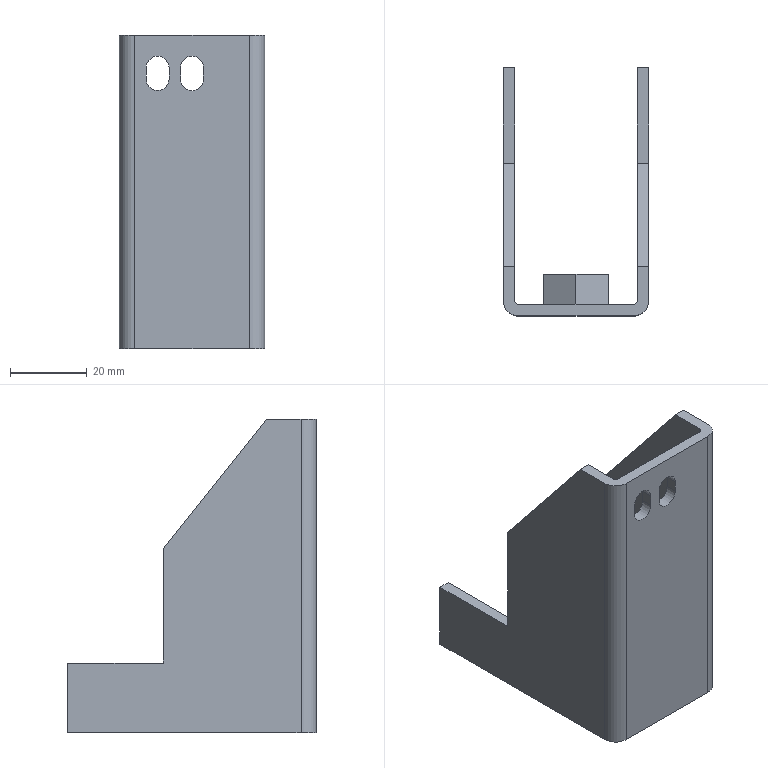Part | NX | features EXTRUDE 4, DATUM_CSYS 3, SKETCH 3, EXTRACT_DATUM_PLANE 1, UNITE 1 | 1 solid | 37 faces | box 38 x 65 x 82 mm | volume 28298 mm3 | plane 28 | cylinder 9 | commonest cylinder face diameters 6 x4 2 x2 8 x2 8.5 x1
STEP:
#1=CARTESIAN_POINT('',(-3.,-29.5,58.5));
#2=VERTEX_POINT('',#1);
#3=CARTESIAN_POINT('',(-3.,-29.5,61.5));
#4=VERTEX_POINT('',#3);
#5=CARTESIAN_POINT('',(-3.,-29.5,58.5));
#6=DIRECTION('',(0.,0.,1.));
#7=VECTOR('',#6,1000.);
#8=LINE('',#5,#7);
#9=EDGE_CURVE('',#2,#4,#8,.T.);
#10=ORIENTED_EDGE('',*,*,#9,.F.);
#11=CARTESIAN_POINT('',(3.,-29.5,58.5));
#12=VERTEX_POINT('',#11);
#13=CARTESIAN_POINT('',(0.,-29.5,58.5));
#14=DIRECTION('',(0.,1.,0.));
#15=DIRECTION('',(-1.,0.,0.));
#16=AXIS2_PLACEMENT_3D('',#13,#14,#15);
#17=CIRCLE('',#16,3.);
#18=EDGE_CURVE('',#12,#2,#17,.T.);
#19=ORIENTED_EDGE('',*,*,#18,.F.);
#20=CARTESIAN_POINT('',(3.,-29.5,61.5));
#21=VERTEX_POINT('',#20);
#22=CARTESIAN_POINT('',(3.,-29.5,61.5));
#23=DIRECTION('',(0.,0.,-1.));
#24=VECTOR('',#23,1000.);
#25=LINE('',#22,#24);
#26=EDGE_CURVE('',#21,#12,#25,.T.);
#27=ORIENTED_EDGE('',*,*,#26,.F.);
#28=CARTESIAN_POINT('',(0.,-29.5,61.5));
#29=DIRECTION('',(0.,1.,0.));
#30=DIRECTION('',(1.,0.,0.));
#31=AXIS2_PLACEMENT_3D('',#28,#29,#30);
#32=CIRCLE('',#31,3.);
#33=EDGE_CURVE('',#4,#21,#32,.T.);
#34=ORIENTED_EDGE('',*,*,#33,.F.);
#35=EDGE_LOOP('',(#10,#19,#27,#34));
#36=FACE_BOUND('',#35,.T.);
#37=CARTESIAN_POINT('',(-12.,-29.5,58.5));
#38=VERTEX_POINT('',#37);
#39=CARTESIAN_POINT('',(-12.,-29.5,61.5));
#40=VERTEX_POINT('',#39);
#41=CARTESIAN_POINT('',(-12.,-29.5,58.5));
#42=DIRECTION('',(0.,0.,1.));
#43=VECTOR('',#42,1000.);
#44=LINE('',#41,#43);
#45=EDGE_CURVE('',#38,#40,#44,.T.);
#46=ORIENTED_EDGE('',*,*,#45,.F.);
#47=CARTESIAN_POINT('',(-6.,-29.5,58.5));
#48=VERTEX_POINT('',#47);
#49=CARTESIAN_POINT('',(-9.,-29.5,58.5));
#50=DIRECTION('',(0.,1.,0.));
#51=DIRECTION('',(-1.,0.,0.));
#52=AXIS2_PLACEMENT_3D('',#49,#50,#51);
#53=CIRCLE('',#52,3.);
#54=EDGE_CURVE('',#48,#38,#53,.T.);
#55=ORIENTED_EDGE('',*,*,#54,.F.);
#56=CARTESIAN_POINT('',(-6.,-29.5,61.5));
#57=VERTEX_POINT('',#56);
#58=CARTESIAN_POINT('',(-6.,-29.5,61.5));
#59=DIRECTION('',(0.,0.,-1.));
#60=VECTOR('',#59,1000.);
#61=LINE('',#58,#60);
#62=EDGE_CURVE('',#57,#48,#61,.T.);
#63=ORIENTED_EDGE('',*,*,#62,.F.);
#64=CARTESIAN_POINT('',(-9.,-29.5,61.5));
#65=DIRECTION('',(0.,1.,0.));
#66=DIRECTION('',(1.,0.,0.));
#67=AXIS2_PLACEMENT_3D('',#64,#65,#66);
#68=CIRCLE('',#67,3.);
#69=EDGE_CURVE('',#40,#57,#68,.T.);
#70=ORIENTED_EDGE('',*,*,#69,.F.);
#71=EDGE_LOOP('',(#46,#55,#63,#70));
#72=FACE_BOUND('',#71,.T.);
#73=CARTESIAN_POINT('',(15.,-29.5,70.));
#74=VERTEX_POINT('',#73);
#75=CARTESIAN_POINT('',(-15.,-29.5,70.));
#76=VERTEX_POINT('',#75);
#77=CARTESIAN_POINT('',(15.,-29.5,70.));
#78=DIRECTION('',(-1.,0.,0.));
#79=VECTOR('',#78,1000.);
#80=LINE('',#77,#79);
#81=EDGE_CURVE('',#74,#76,#80,.T.);
#82=ORIENTED_EDGE('',*,*,#81,.F.);
#83=CARTESIAN_POINT('',(15.,-29.5,-12.));
#84=VERTEX_POINT('',#83);
#85=CARTESIAN_POINT('',(15.,-29.5,-12.));
#86=DIRECTION('',(0.,0.,1.));
#87=VECTOR('',#86,1000.);
#88=LINE('',#85,#87);
#89=EDGE_CURVE('',#84,#74,#88,.T.);
#90=ORIENTED_EDGE('',*,*,#89,.F.);
#91=CARTESIAN_POINT('',(-15.,-29.5,-12.));
#92=VERTEX_POINT('',#91);
#93=CARTESIAN_POINT('',(15.,-29.5,-12.));
#94=DIRECTION('',(-1.,0.,0.));
#95=VECTOR('',#94,1000.);
#96=LINE('',#93,#95);
#97=EDGE_CURVE('',#84,#92,#96,.T.);
#98=ORIENTED_EDGE('',*,*,#97,.T.);
#99=CARTESIAN_POINT('',(-15.,-29.5,-12.));
#100=DIRECTION('',(0.,0.,1.));
#101=VECTOR('',#100,1000.);
#102=LINE('',#99,#101);
#103=EDGE_CURVE('',#92,#76,#102,.T.);
#104=ORIENTED_EDGE('',*,*,#103,.T.);
#105=EDGE_LOOP('',(#82,#90,#98,#104));
#106=FACE_BOUND('',#105,.T.);
#107=CARTESIAN_POINT('',(8.5,-29.5,4.907));
#108=VERTEX_POINT('',#107);
#109=CARTESIAN_POINT('',(8.5,-29.5,-4.907));
#110=VERTEX_POINT('',#109);
#111=CARTESIAN_POINT('',(8.5,-29.5,4.907));
#112=DIRECTION('',(0.,0.,-1.));
#113=VECTOR('',#112,1000.);
#114=LINE('',#111,#113);
#115=EDGE_CURVE('',#108,#110,#114,.T.);
#116=ORIENTED_EDGE('',*,*,#115,.F.);
#117=CARTESIAN_POINT('',(0.,-29.5,9.815));
#118=VERTEX_POINT('',#117);
#119=CARTESIAN_POINT('',(0.,-29.5,9.815));
#120=DIRECTION('',(0.866,0.,-0.5));
#121=VECTOR('',#120,1000.);
#122=LINE('',#119,#121);
#123=EDGE_CURVE('',#118,#108,#122,.T.);
#124=ORIENTED_EDGE('',*,*,#123,.F.);
#125=CARTESIAN_POINT('',(-8.5,-29.5,4.907));
#126=VERTEX_POINT('',#125);
#127=CARTESIAN_POINT('',(-8.5,-29.5,4.907));
#128=DIRECTION('',(0.866,0.,0.5));
#129=VECTOR('',#128,1000.);
#130=LINE('',#127,#129);
#131=EDGE_CURVE('',#126,#118,#130,.T.);
#132=ORIENTED_EDGE('',*,*,#131,.F.);
#133=CARTESIAN_POINT('',(-8.5,-29.5,-4.907));
#134=VERTEX_POINT('',#133);
#135=CARTESIAN_POINT('',(-8.5,-29.5,-4.907));
#136=DIRECTION('',(0.,0.,1.));
#137=VECTOR('',#136,1000.);
#138=LINE('',#135,#137);
#139=EDGE_CURVE('',#134,#126,#138,.T.);
#140=ORIENTED_EDGE('',*,*,#139,.F.);
#141=CARTESIAN_POINT('',(0.,-29.5,-9.815));
#142=VERTEX_POINT('',#141);
#143=CARTESIAN_POINT('',(0.,-29.5,-9.815));
#144=DIRECTION('',(-0.866,0.,0.5));
#145=VECTOR('',#144,1000.);
#146=LINE('',#143,#145);
#147=EDGE_CURVE('',#142,#134,#146,.T.);
#148=ORIENTED_EDGE('',*,*,#147,.F.);
#149=CARTESIAN_POINT('',(8.5,-29.5,-4.907));
#150=DIRECTION('',(-0.866,0.,-0.5));
#151=VECTOR('',#150,1000.);
#152=LINE('',#149,#151);
#153=EDGE_CURVE('',#110,#142,#152,.T.);
#154=ORIENTED_EDGE('',*,*,#153,.F.);
#155=EDGE_LOOP('',(#116,#124,#132,#140,#148,#154));
#156=FACE_BOUND('',#155,.T.);
#157=CARTESIAN_POINT('',(15.,-29.5,-12.));
#158=DIRECTION('',(0.,1.,0.));
#159=DIRECTION('',(0.,0.,1.));
#160=AXIS2_PLACEMENT_3D('',#157,#158,#159);
#161=PLANE('',#160);
#162=ADVANCED_FACE('',(#36,#72,#106,#156),#161,.T.);
#163=CARTESIAN_POINT('',(-19.,-28.5,70.));
#164=VERTEX_POINT('',#163);
#165=CARTESIAN_POINT('',(-15.,-32.5,70.));
#166=VERTEX_POINT('',#165);
#167=CARTESIAN_POINT('',(-15.,-28.5,70.));
#168=DIRECTION('',(0.,0.,1.));
#169=DIRECTION('',(-1.,0.,0.));
#170=AXIS2_PLACEMENT_3D('',#167,#168,#169);
#171=CIRCLE('',#170,4.);
#172=EDGE_CURVE('',#164,#166,#171,.T.);
#173=ORIENTED_EDGE('',*,*,#172,.F.);
#174=CARTESIAN_POINT('',(-19.,-28.5,-12.));
#175=VERTEX_POINT('',#174);
#176=CARTESIAN_POINT('',(-19.,-28.5,-12.));
#177=DIRECTION('',(0.,0.,1.));
#178=VECTOR('',#177,1000.);
#179=LINE('',#176,#178);
#180=EDGE_CURVE('',#175,#164,#179,.T.);
#181=ORIENTED_EDGE('',*,*,#180,.F.);
#182=CARTESIAN_POINT('',(-15.,-32.5,-12.));
#183=VERTEX_POINT('',#182);
#184=CARTESIAN_POINT('',(-15.,-28.5,-12.));
#185=DIRECTION('',(0.,0.,1.));
#186=DIRECTION('',(-1.,0.,0.));
#187=AXIS2_PLACEMENT_3D('',#184,#185,#186);
#188=CIRCLE('',#187,4.);
#189=EDGE_CURVE('',#175,#183,#188,.T.);
#190=ORIENTED_EDGE('',*,*,#189,.T.);
#191=CARTESIAN_POINT('',(-15.,-32.5,-12.));
#192=DIRECTION('',(0.,0.,1.));
#193=VECTOR('',#192,1000.);
#194=LINE('',#191,#193);
#195=EDGE_CURVE('',#183,#166,#194,.T.);
#196=ORIENTED_EDGE('',*,*,#195,.T.);
#197=EDGE_LOOP('',(#173,#181,#190,#196));
#198=FACE_BOUND('',#197,.T.);
#199=CARTESIAN_POINT('',(-15.,-28.5,-12.));
#200=DIRECTION('',(0.,0.,1.));
#201=DIRECTION('',(1.,0.,0.));
#202=AXIS2_PLACEMENT_3D('',#199,#200,#201);
#203=CYLINDRICAL_SURFACE('',#202,4.);
#204=ADVANCED_FACE('',(#198),#203,.T.);
#205=CARTESIAN_POINT('',(-3.,-32.5,61.5));
#206=VERTEX_POINT('',#205);
#207=CARTESIAN_POINT('',(-3.,-32.5,58.5));
#208=VERTEX_POINT('',#207);
#209=CARTESIAN_POINT('',(-3.,-32.5,-12.));
#210=DIRECTION('',(0.,0.,-1.));
#211=VECTOR('',#210,1000.);
#212=LINE('',#209,#211);
#213=EDGE_CURVE('',#206,#208,#212,.T.);
#214=ORIENTED_EDGE('',*,*,#213,.F.);
#215=CARTESIAN_POINT('',(3.,-32.5,61.5));
#216=VERTEX_POINT('',#215);
#217=CARTESIAN_POINT('',(0.,-32.5,61.5));
#218=DIRECTION('',(0.,-1.,0.));
#219=DIRECTION('',(0.,0.,-1.));
#220=AXIS2_PLACEMENT_3D('',#217,#218,#219);
#221=CIRCLE('',#220,3.);
#222=EDGE_CURVE('',#216,#206,#221,.T.);
#223=ORIENTED_EDGE('',*,*,#222,.F.);
#224=CARTESIAN_POINT('',(3.,-32.5,58.5));
#225=VERTEX_POINT('',#224);
#226=CARTESIAN_POINT('',(3.,-32.5,-12.));
#227=DIRECTION('',(0.,0.,1.));
#228=VECTOR('',#227,1000.);
#229=LINE('',#226,#228);
#230=EDGE_CURVE('',#225,#216,#229,.T.);
#231=ORIENTED_EDGE('',*,*,#230,.F.);
#232=CARTESIAN_POINT('',(0.,-32.5,58.5));
#233=DIRECTION('',(0.,-1.,0.));
#234=DIRECTION('',(0.,0.,-1.));
#235=AXIS2_PLACEMENT_3D('',#232,#233,#234);
#236=CIRCLE('',#235,3.);
#237=EDGE_CURVE('',#208,#225,#236,.T.);
#238=ORIENTED_EDGE('',*,*,#237,.F.);
#239=EDGE_LOOP('',(#214,#223,#231,#238));
#240=FACE_BOUND('',#239,.T.);
#241=CARTESIAN_POINT('',(-12.,-32.5,61.5));
#242=VERTEX_POINT('',#241);
#243=CARTESIAN_POINT('',(-12.,-32.5,58.5));
#244=VERTEX_POINT('',#243);
#245=CARTESIAN_POINT('',(-12.,-32.5,-12.));
#246=DIRECTION('',(0.,0.,-1.));
#247=VECTOR('',#246,1000.);
#248=LINE('',#245,#247);
#249=EDGE_CURVE('',#242,#244,#248,.T.);
#250=ORIENTED_EDGE('',*,*,#249,.F.);
#251=CARTESIAN_POINT('',(-6.,-32.5,61.5));
#252=VERTEX_POINT('',#251);
#253=CARTESIAN_POINT('',(-9.,-32.5,61.5));
#254=DIRECTION('',(0.,-1.,0.));
#255=DIRECTION('',(0.,0.,-1.));
#256=AXIS2_PLACEMENT_3D('',#253,#254,#255);
#257=CIRCLE('',#256,3.);
#258=EDGE_CURVE('',#252,#242,#257,.T.);
#259=ORIENTED_EDGE('',*,*,#258,.F.);
#260=CARTESIAN_POINT('',(-6.,-32.5,58.5));
#261=VERTEX_POINT('',#260);
#262=CARTESIAN_POINT('',(-6.,-32.5,-12.));
#263=DIRECTION('',(0.,0.,1.));
#264=VECTOR('',#263,1000.);
#265=LINE('',#262,#264);
#266=EDGE_CURVE('',#261,#252,#265,.T.);
#267=ORIENTED_EDGE('',*,*,#266,.F.);
#268=CARTESIAN_POINT('',(-9.,-32.5,58.5));
#269=DIRECTION('',(0.,-1.,0.));
#270=DIRECTION('',(0.,0.,-1.));
#271=AXIS2_PLACEMENT_3D('',#268,#269,#270);
#272=CIRCLE('',#271,3.);
#273=EDGE_CURVE('',#244,#261,#272,.T.);
#274=ORIENTED_EDGE('',*,*,#273,.F.);
#275=EDGE_LOOP('',(#250,#259,#267,#274));
#276=FACE_BOUND('',#275,.T.);
#277=CARTESIAN_POINT('',(15.,-32.5,70.));
#278=VERTEX_POINT('',#277);
#279=CARTESIAN_POINT('',(-15.,-32.5,70.));
#280=DIRECTION('',(1.,0.,0.));
#281=VECTOR('',#280,1000.);
#282=LINE('',#279,#281);
#283=EDGE_CURVE('',#166,#278,#282,.T.);
#284=ORIENTED_EDGE('',*,*,#283,.F.);
#285=ORIENTED_EDGE('',*,*,#195,.F.);
#286=CARTESIAN_POINT('',(15.,-32.5,-12.));
#287=VERTEX_POINT('',#286);
#288=CARTESIAN_POINT('',(-15.,-32.5,-12.));
#289=DIRECTION('',(1.,0.,0.));
#290=VECTOR('',#289,1000.);
#291=LINE('',#288,#290);
#292=EDGE_CURVE('',#183,#287,#291,.T.);
#293=ORIENTED_EDGE('',*,*,#292,.T.);
#294=CARTESIAN_POINT('',(15.,-32.5,-12.));
#295=DIRECTION('',(0.,0.,1.));
#296=VECTOR('',#295,1000.);
#297=LINE('',#294,#296);
#298=EDGE_CURVE('',#287,#278,#297,.T.);
#299=ORIENTED_EDGE('',*,*,#298,.T.);
#300=EDGE_LOOP('',(#284,#285,#293,#299));
#301=FACE_BOUND('',#300,.T.);
#302=CARTESIAN_POINT('',(-15.,-32.5,-12.));
#303=DIRECTION('',(0.,-1.,0.));
#304=DIRECTION('',(0.,0.,-1.));
#305=AXIS2_PLACEMENT_3D('',#302,#303,#304);
#306=PLANE('',#305);
#307=ADVANCED_FACE('',(#240,#276,#301),#306,.T.);
#308=CARTESIAN_POINT('',(19.,-28.5,70.));
#309=VERTEX_POINT('',#308);
#310=CARTESIAN_POINT('',(15.,-28.5,70.));
#311=DIRECTION('',(0.,0.,1.));
#312=DIRECTION('',(0.,-1.,0.));
#313=AXIS2_PLACEMENT_3D('',#310,#311,#312);
#314=CIRCLE('',#313,4.);
#315=EDGE_CURVE('',#278,#309,#314,.T.);
#316=ORIENTED_EDGE('',*,*,#315,.F.);
#317=ORIENTED_EDGE('',*,*,#298,.F.);
#318=CARTESIAN_POINT('',(19.,-28.5,-12.));
#319=VERTEX_POINT('',#318);
#320=CARTESIAN_POINT('',(15.,-28.5,-12.));
#321=DIRECTION('',(0.,0.,1.));
#322=DIRECTION('',(0.,-1.,0.));
#323=AXIS2_PLACEMENT_3D('',#320,#321,#322);
#324=CIRCLE('',#323,4.);
#325=EDGE_CURVE('',#287,#319,#324,.T.);
#326=ORIENTED_EDGE('',*,*,#325,.T.);
#327=CARTESIAN_POINT('',(19.,-28.5,-12.));
#328=DIRECTION('',(0.,0.,1.));
#329=VECTOR('',#328,1000.);
#330=LINE('',#327,#329);
#331=EDGE_CURVE('',#319,#309,#330,.T.);
#332=ORIENTED_EDGE('',*,*,#331,.T.);
#333=EDGE_LOOP('',(#316,#317,#326,#332));
#334=FACE_BOUND('',#333,.T.);
#335=CARTESIAN_POINT('',(15.,-28.5,-12.));
#336=DIRECTION('',(0.,0.,1.));
#337=DIRECTION('',(1.,0.,0.));
#338=AXIS2_PLACEMENT_3D('',#335,#336,#337);
#339=CYLINDRICAL_SURFACE('',#338,4.);
#340=ADVANCED_FACE('',(#334),#339,.T.);
#341=CARTESIAN_POINT('',(19.,7.5,6.25));
#342=VERTEX_POINT('',#341);
#343=CARTESIAN_POINT('',(19.,32.5,6.25));
#344=VERTEX_POINT('',#343);
#345=CARTESIAN_POINT('',(19.,7.5,6.25));
#346=DIRECTION('',(0.,1.,0.));
#347=VECTOR('',#346,1000.);
#348=LINE('',#345,#347);
#349=EDGE_CURVE('',#342,#344,#348,.T.);
#350=ORIENTED_EDGE('',*,*,#349,.F.);
#351=CARTESIAN_POINT('',(19.,7.5,36.25));
#352=VERTEX_POINT('',#351);
#353=CARTESIAN_POINT('',(19.,7.5,-12.));
#354=DIRECTION('',(0.,0.,-1.));
#355=VECTOR('',#354,1000.);
#356=LINE('',#353,#355);
#357=EDGE_CURVE('',#352,#342,#356,.T.);
#358=ORIENTED_EDGE('',*,*,#357,.F.);
#359=CARTESIAN_POINT('',(19.,-19.5,70.));
#360=VERTEX_POINT('',#359);
#361=CARTESIAN_POINT('',(19.,31.037,6.829));
#362=DIRECTION('',(0.,0.6247,-0.7809));
#363=VECTOR('',#362,1000.);
#364=LINE('',#361,#363);
#365=EDGE_CURVE('',#360,#352,#364,.T.);
#366=ORIENTED_EDGE('',*,*,#365,.F.);
#367=CARTESIAN_POINT('',(19.,7.5,70.));
#368=DIRECTION('',(0.,1.,0.));
#369=VECTOR('',#368,1000.);
#370=LINE('',#367,#369);
#371=EDGE_CURVE('',#309,#360,#370,.T.);
#372=ORIENTED_EDGE('',*,*,#371,.F.);
#373=ORIENTED_EDGE('',*,*,#331,.F.);
#374=CARTESIAN_POINT('',(19.,32.5,-12.));
#375=VERTEX_POINT('',#374);
#376=CARTESIAN_POINT('',(19.,-28.5,-12.));
#377=DIRECTION('',(0.,1.,0.));
#378=VECTOR('',#377,1000.);
#379=LINE('',#376,#378);
#380=EDGE_CURVE('',#319,#375,#379,.T.);
#381=ORIENTED_EDGE('',*,*,#380,.T.);
#382=CARTESIAN_POINT('',(19.,32.5,-12.));
#383=DIRECTION('',(0.,0.,1.));
#384=VECTOR('',#383,1000.);
#385=LINE('',#382,#384);
#386=EDGE_CURVE('',#375,#344,#385,.T.);
#387=ORIENTED_EDGE('',*,*,#386,.T.);
#388=EDGE_LOOP('',(#350,#358,#366,#372,#373,#381,#387));
#389=FACE_BOUND('',#388,.T.);
#390=CARTESIAN_POINT('',(19.,7.5,-12.));
#391=DIRECTION('',(1.,0.,0.));
#392=DIRECTION('',(0.,0.,-1.));
#393=AXIS2_PLACEMENT_3D('',#390,#391,#392);
#394=PLANE('',#393);
#395=ADVANCED_FACE('',(#389),#394,.T.);
#396=CARTESIAN_POINT('',(16.,32.5,6.25));
#397=VERTEX_POINT('',#396);
#398=CARTESIAN_POINT('',(19.,32.5,6.25));
#399=DIRECTION('',(-1.,0.,0.));
#400=VECTOR('',#399,1000.);
#401=LINE('',#398,#400);
#402=EDGE_CURVE('',#344,#397,#401,.T.);
#403=ORIENTED_EDGE('',*,*,#402,.F.);
#404=ORIENTED_EDGE('',*,*,#386,.F.);
#405=CARTESIAN_POINT('',(16.,32.5,-12.));
#406=VERTEX_POINT('',#405);
#407=CARTESIAN_POINT('',(19.,32.5,-12.));
#408=DIRECTION('',(-1.,0.,0.));
#409=VECTOR('',#408,1000.);
#410=LINE('',#407,#409);
#411=EDGE_CURVE('',#375,#406,#410,.T.);
#412=ORIENTED_EDGE('',*,*,#411,.T.);
#413=CARTESIAN_POINT('',(16.,32.5,-12.));
#414=DIRECTION('',(0.,0.,1.));
#415=VECTOR('',#414,1000.);
#416=LINE('',#413,#415);
#417=EDGE_CURVE('',#406,#397,#416,.T.);
#418=ORIENTED_EDGE('',*,*,#417,.T.);
#419=EDGE_LOOP('',(#403,#404,#412,#418));
#420=FACE_BOUND('',#419,.T.);
#421=CARTESIAN_POINT('',(19.,32.5,-12.));
#422=DIRECTION('',(0.,1.,0.));
#423=DIRECTION('',(0.,0.,1.));
#424=AXIS2_PLACEMENT_3D('',#421,#422,#423);
#425=PLANE('',#424);
#426=ADVANCED_FACE('',(#420),#425,.T.);
#427=CARTESIAN_POINT('',(16.,7.5,6.25));
#428=VERTEX_POINT('',#427);
#429=CARTESIAN_POINT('',(16.,-19.5,6.25));
#430=DIRECTION('',(0.,-1.,0.));
#431=VECTOR('',#430,1000.);
#432=LINE('',#429,#431);
#433=EDGE_CURVE('',#397,#428,#432,.T.);
#434=ORIENTED_EDGE('',*,*,#433,.F.);
#435=ORIENTED_EDGE('',*,*,#417,.F.);
#436=CARTESIAN_POINT('',(16.,-28.5,-12.));
#437=VERTEX_POINT('',#436);
#438=CARTESIAN_POINT('',(16.,32.5,-12.));
#439=DIRECTION('',(0.,-1.,0.));
#440=VECTOR('',#439,1000.);
#441=LINE('',#438,#440);
#442=EDGE_CURVE('',#406,#437,#441,.T.);
#443=ORIENTED_EDGE('',*,*,#442,.T.);
#444=CARTESIAN_POINT('',(16.,-28.5,70.));
#445=VERTEX_POINT('',#444);
#446=CARTESIAN_POINT('',(16.,-28.5,-12.));
#447=DIRECTION('',(0.,0.,1.));
#448=VECTOR('',#447,1000.);
#449=LINE('',#446,#448);
#450=EDGE_CURVE('',#437,#445,#449,.T.);
#451=ORIENTED_EDGE('',*,*,#450,.T.);
#452=CARTESIAN_POINT('',(16.,-19.5,70.));
#453=VERTEX_POINT('',#452);
#454=CARTESIAN_POINT('',(16.,-19.5,70.));
#455=DIRECTION('',(0.,-1.,0.));
#456=VECTOR('',#455,1000.);
#457=LINE('',#454,#456);
#458=EDGE_CURVE('',#453,#445,#457,.T.);
#459=ORIENTED_EDGE('',*,*,#458,.F.);
#460=CARTESIAN_POINT('',(16.,7.5,36.25));
#461=VERTEX_POINT('',#460);
#462=CARTESIAN_POINT('',(16.,20.5,20.));
#463=DIRECTION('',(0.,-0.6247,0.7809));
#464=VECTOR('',#463,1000.);
#465=LINE('',#462,#464);
#466=EDGE_CURVE('',#461,#453,#465,.T.);
#467=ORIENTED_EDGE('',*,*,#466,.F.);
#468=CARTESIAN_POINT('',(16.,7.5,-12.));
#469=DIRECTION('',(0.,0.,1.));
#470=VECTOR('',#469,1000.);
#471=LINE('',#468,#470);
#472=EDGE_CURVE('',#428,#461,#471,.T.);
#473=ORIENTED_EDGE('',*,*,#472,.F.);
#474=EDGE_LOOP('',(#434,#435,#443,#451,#459,#467,#473));
#475=FACE_BOUND('',#474,.T.);
#476=CARTESIAN_POINT('',(16.,-19.5,-12.));
#477=DIRECTION('',(-1.,0.,0.));
#478=DIRECTION('',(0.,0.,1.));
#479=AXIS2_PLACEMENT_3D('',#476,#477,#478);
#480=PLANE('',#479);
#481=ADVANCED_FACE('',(#475),#480,.T.);
#482=CARTESIAN_POINT('',(15.,-28.5,70.));
#483=DIRECTION('',(0.,0.,-1.));
#484=DIRECTION('',(1.,0.,0.));
#485=AXIS2_PLACEMENT_3D('',#482,#483,#484);
#486=CIRCLE('',#485,1.);
#487=EDGE_CURVE('',#445,#74,#486,.T.);
#488=ORIENTED_EDGE('',*,*,#487,.F.);
#489=ORIENTED_EDGE('',*,*,#450,.F.);
#490=CARTESIAN_POINT('',(15.,-28.5,-12.));
#491=DIRECTION('',(0.,0.,-1.));
#492=DIRECTION('',(1.,0.,0.));
#493=AXIS2_PLACEMENT_3D('',#490,#491,#492);
#494=CIRCLE('',#493,1.);
#495=EDGE_CURVE('',#437,#84,#494,.T.);
#496=ORIENTED_EDGE('',*,*,#495,.T.);
#497=ORIENTED_EDGE('',*,*,#89,.T.);
#498=EDGE_LOOP('',(#488,#489,#496,#497));
#499=FACE_BOUND('',#498,.T.);
#500=CARTESIAN_POINT('',(15.,-28.5,-12.));
#501=DIRECTION('',(0.,0.,1.));
#502=DIRECTION('',(1.,0.,0.));
#503=AXIS2_PLACEMENT_3D('',#500,#501,#502);
#504=CYLINDRICAL_SURFACE('',#503,1.);
#505=ADVANCED_FACE('',(#499),#504,.F.);
#506=CARTESIAN_POINT('',(-16.,-28.5,70.));
#507=VERTEX_POINT('',#506);
#508=CARTESIAN_POINT('',(-15.,-28.5,70.));
#509=DIRECTION('',(0.,0.,-1.));
#510=DIRECTION('',(0.,-1.,0.));
#511=AXIS2_PLACEMENT_3D('',#508,#509,#510);
#512=CIRCLE('',#511,1.);
#513=EDGE_CURVE('',#76,#507,#512,.T.);
#514=ORIENTED_EDGE('',*,*,#513,.F.);
#515=ORIENTED_EDGE('',*,*,#103,.F.);
#516=CARTESIAN_POINT('',(-16.,-28.5,-12.));
#517=VERTEX_POINT('',#516);
#518=CARTESIAN_POINT('',(-15.,-28.5,-12.));
#519=DIRECTION('',(0.,0.,-1.));
#520=DIRECTION('',(0.,-1.,0.));
#521=AXIS2_PLACEMENT_3D('',#518,#519,#520);
#522=CIRCLE('',#521,1.);
#523=EDGE_CURVE('',#92,#517,#522,.T.);
#524=ORIENTED_EDGE('',*,*,#523,.T.);
#525=CARTESIAN_POINT('',(-16.,-28.5,-12.));
#526=DIRECTION('',(0.,0.,1.));
#527=VECTOR('',#526,1000.);
#528=LINE('',#525,#527);
#529=EDGE_CURVE('',#517,#507,#528,.T.);
#530=ORIENTED_EDGE('',*,*,#529,.T.);
#531=EDGE_LOOP('',(#514,#515,#524,#530));
#532=FACE_BOUND('',#531,.T.);
#533=CARTESIAN_POINT('',(-15.,-28.5,-12.));
#534=DIRECTION('',(0.,0.,1.));
#535=DIRECTION('',(1.,0.,0.));
#536=AXIS2_PLACEMENT_3D('',#533,#534,#535);
#537=CYLINDRICAL_SURFACE('',#536,1.);
#538=ADVANCED_FACE('',(#532),#537,.F.);
#539=CARTESIAN_POINT('',(-16.,7.5,6.25));
#540=VERTEX_POINT('',#539);
#541=CARTESIAN_POINT('',(-16.,32.5,6.25));
#542=VERTEX_POINT('',#541);
#543=CARTESIAN_POINT('',(-16.,7.5,6.25));
#544=DIRECTION('',(0.,1.,0.));
#545=VECTOR('',#544,1000.);
#546=LINE('',#543,#545);
#547=EDGE_CURVE('',#540,#542,#546,.T.);
#548=ORIENTED_EDGE('',*,*,#547,.F.);
#549=CARTESIAN_POINT('',(-16.,7.5,36.25));
#550=VERTEX_POINT('',#549);
#551=CARTESIAN_POINT('',(-16.,7.5,-12.));
#552=DIRECTION('',(0.,0.,-1.));
#553=VECTOR('',#552,1000.);
#554=LINE('',#551,#553);
#555=EDGE_CURVE('',#550,#540,#554,.T.);
#556=ORIENTED_EDGE('',*,*,#555,.F.);
#557=CARTESIAN_POINT('',(-16.,-19.5,70.));
#558=VERTEX_POINT('',#557);
#559=CARTESIAN_POINT('',(-16.,31.037,6.829));
#560=DIRECTION('',(0.,0.6247,-0.7809));
#561=VECTOR('',#560,1000.);
#562=LINE('',#559,#561);
#563=EDGE_CURVE('',#558,#550,#562,.T.);
#564=ORIENTED_EDGE('',*,*,#563,.F.);
#565=CARTESIAN_POINT('',(-16.,7.5,70.));
#566=DIRECTION('',(0.,1.,0.));
#567=VECTOR('',#566,1000.);
#568=LINE('',#565,#567);
#569=EDGE_CURVE('',#507,#558,#568,.T.);
#570=ORIENTED_EDGE('',*,*,#569,.F.);
#571=ORIENTED_EDGE('',*,*,#529,.F.);
#572=CARTESIAN_POINT('',(-16.,32.5,-12.));
#573=VERTEX_POINT('',#572);
#574=CARTESIAN_POINT('',(-16.,-28.5,-12.));
#575=DIRECTION('',(0.,1.,0.));
#576=VECTOR('',#575,1000.);
#577=LINE('',#574,#576);
#578=EDGE_CURVE('',#517,#573,#577,.T.);
#579=ORIENTED_EDGE('',*,*,#578,.T.);
#580=CARTESIAN_POINT('',(-16.,32.5,-12.));
#581=DIRECTION('',(0.,0.,1.));
#582=VECTOR('',#581,1000.);
#583=LINE('',#580,#582);
#584=EDGE_CURVE('',#573,#542,#583,.T.);
#585=ORIENTED_EDGE('',*,*,#584,.T.);
#586=EDGE_LOOP('',(#548,#556,#564,#570,#571,#579,#585));
#587=FACE_BOUND('',#586,.T.);
#588=CARTESIAN_POINT('',(-16.,7.5,-12.));
#589=DIRECTION('',(1.,0.,0.));
#590=DIRECTION('',(0.,0.,-1.));
#591=AXIS2_PLACEMENT_3D('',#588,#589,#590);
#592=PLANE('',#591);
#593=ADVANCED_FACE('',(#587),#592,.T.);
#594=CARTESIAN_POINT('',(-19.,32.5,6.25));
#595=VERTEX_POINT('',#594);
#596=CARTESIAN_POINT('',(-16.,32.5,6.25));
#597=DIRECTION('',(-1.,0.,0.));
#598=VECTOR('',#597,1000.);
#599=LINE('',#596,#598);
#600=EDGE_CURVE('',#542,#595,#599,.T.);
#601=ORIENTED_EDGE('',*,*,#600,.F.);
#602=ORIENTED_EDGE('',*,*,#584,.F.);
#603=CARTESIAN_POINT('',(-19.,32.5,-12.));
#604=VERTEX_POINT('',#603);
#605=CARTESIAN_POINT('',(-16.,32.5,-12.));
#606=DIRECTION('',(-1.,0.,0.));
#607=VECTOR('',#606,1000.);
#608=LINE('',#605,#607);
#609=EDGE_CURVE('',#573,#604,#608,.T.);
#610=ORIENTED_EDGE('',*,*,#609,.T.);
#611=CARTESIAN_POINT('',(-19.,32.5,-12.));
#612=DIRECTION('',(0.,0.,1.));
#613=VECTOR('',#612,1000.);
#614=LINE('',#611,#613);
#615=EDGE_CURVE('',#604,#595,#614,.T.);
#616=ORIENTED_EDGE('',*,*,#615,.T.);
#617=EDGE_LOOP('',(#601,#602,#610,#616));
#618=FACE_BOUND('',#617,.T.);
#619=CARTESIAN_POINT('',(-16.,32.5,-12.));
#620=DIRECTION('',(0.,1.,0.));
#621=DIRECTION('',(0.,0.,1.));
#622=AXIS2_PLACEMENT_3D('',#619,#620,#621);
#623=PLANE('',#622);
#624=ADVANCED_FACE('',(#618),#623,.T.);
#625=CARTESIAN_POINT('',(-19.,7.5,6.25));
#626=VERTEX_POINT('',#625);
#627=CARTESIAN_POINT('',(-19.,32.5,6.25));
#628=DIRECTION('',(0.,-1.,0.));
#629=VECTOR('',#628,1000.);
#630=LINE('',#627,#629);
#631=EDGE_CURVE('',#595,#626,#630,.T.);
#632=ORIENTED_EDGE('',*,*,#631,.F.);
#633=ORIENTED_EDGE('',*,*,#615,.F.);
#634=CARTESIAN_POINT('',(-19.,-19.5,-12.));
#635=DIRECTION('',(0.,-1.,0.));
#636=VECTOR('',#635,1000.);
#637=LINE('',#634,#636);
#638=EDGE_CURVE('',#604,#175,#637,.T.);
#639=ORIENTED_EDGE('',*,*,#638,.T.);
#640=ORIENTED_EDGE('',*,*,#180,.T.);
#641=CARTESIAN_POINT('',(-19.,-19.5,70.));
#642=VERTEX_POINT('',#641);
#643=CARTESIAN_POINT('',(-19.,7.5,70.));
#644=DIRECTION('',(0.,-1.,0.));
#645=VECTOR('',#644,1000.);
#646=LINE('',#643,#645);
#647=EDGE_CURVE('',#642,#164,#646,.T.);
#648=ORIENTED_EDGE('',*,*,#647,.F.);
#649=CARTESIAN_POINT('',(-19.,7.5,36.25));
#650=VERTEX_POINT('',#649);
#651=CARTESIAN_POINT('',(-19.,7.5,36.25));
#652=DIRECTION('',(0.,-0.6247,0.7809));
#653=VECTOR('',#652,1000.);
#654=LINE('',#651,#653);
#655=EDGE_CURVE('',#650,#642,#654,.T.);
#656=ORIENTED_EDGE('',*,*,#655,.F.);
#657=CARTESIAN_POINT('',(-19.,7.5,6.25));
#658=DIRECTION('',(0.,0.,1.));
#659=VECTOR('',#658,1000.);
#660=LINE('',#657,#659);
#661=EDGE_CURVE('',#626,#650,#660,.T.);
#662=ORIENTED_EDGE('',*,*,#661,.F.);
#663=EDGE_LOOP('',(#632,#633,#639,#640,#648,#656,#662));
#664=FACE_BOUND('',#663,.T.);
#665=CARTESIAN_POINT('',(-19.,7.5,-12.));
#666=DIRECTION('',(-1.,0.,0.));
#667=DIRECTION('',(0.,0.,1.));
#668=AXIS2_PLACEMENT_3D('',#665,#666,#667);
#669=PLANE('',#668);
#670=ADVANCED_FACE('',(#664),#669,.T.);
#671=ORIENTED_EDGE('',*,*,#638,.F.);
#672=ORIENTED_EDGE('',*,*,#609,.F.);
#673=ORIENTED_EDGE('',*,*,#578,.F.);
#674=ORIENTED_EDGE('',*,*,#523,.F.);
#675=ORIENTED_EDGE('',*,*,#97,.F.);
#676=ORIENTED_EDGE('',*,*,#495,.F.);
#677=ORIENTED_EDGE('',*,*,#442,.F.);
#678=ORIENTED_EDGE('',*,*,#411,.F.);
#679=ORIENTED_EDGE('',*,*,#380,.F.);
#680=ORIENTED_EDGE('',*,*,#325,.F.);
#681=ORIENTED_EDGE('',*,*,#292,.F.);
#682=ORIENTED_EDGE('',*,*,#189,.F.);
#683=EDGE_LOOP('',(#671,#672,#673,#674,#675,#676,#677,#678,#679,#680,#681,#682));
#684=FACE_BOUND('',#683,.T.);
#685=CARTESIAN_POINT('',(-15.,-28.5,-12.));
#686=DIRECTION('',(0.,0.,1.));
#687=DIRECTION('',(1.,0.,0.));
#688=AXIS2_PLACEMENT_3D('',#685,#686,#687);
#689=PLANE('',#688);
#690=ADVANCED_FACE('',(#684),#689,.F.);
#691=CARTESIAN_POINT('',(-15.,-19.5,70.));
#692=DIRECTION('',(1.,0.,0.));
#693=VECTOR('',#692,1000.);
#694=LINE('',#691,#693);
#695=EDGE_CURVE('',#558,#642,#694,.F.);
#696=ORIENTED_EDGE('',*,*,#695,.T.);
#697=ORIENTED_EDGE('',*,*,#647,.T.);
#698=ORIENTED_EDGE('',*,*,#172,.T.);
#699=ORIENTED_EDGE('',*,*,#283,.T.);
#700=ORIENTED_EDGE('',*,*,#315,.T.);
#701=ORIENTED_EDGE('',*,*,#371,.T.);
#702=CARTESIAN_POINT('',(867.75,-19.5,70.));
#703=DIRECTION('',(-1.,0.,0.));
#704=VECTOR('',#703,1000.);
#705=LINE('',#702,#704);
#706=EDGE_CURVE('',#360,#453,#705,.T.);
#707=ORIENTED_EDGE('',*,*,#706,.T.);
#708=ORIENTED_EDGE('',*,*,#458,.T.);
#709=ORIENTED_EDGE('',*,*,#487,.T.);
#710=ORIENTED_EDGE('',*,*,#81,.T.);
#711=ORIENTED_EDGE('',*,*,#513,.T.);
#712=ORIENTED_EDGE('',*,*,#569,.T.);
#713=EDGE_LOOP('',(#696,#697,#698,#699,#700,#701,#707,#708,#709,#710,#711,#712));
#714=FACE_BOUND('',#713,.T.);
#715=CARTESIAN_POINT('',(-15.,-28.5,70.));
#716=DIRECTION('',(0.,0.,1.));
#717=DIRECTION('',(1.,0.,0.));
#718=AXIS2_PLACEMENT_3D('',#715,#716,#717);
#719=PLANE('',#718);
#720=ADVANCED_FACE('',(#714),#719,.T.);
#721=ORIENTED_EDGE('',*,*,#365,.T.);
#722=CARTESIAN_POINT('',(867.75,7.5,36.25));
#723=DIRECTION('',(-1.,0.,0.));
#724=VECTOR('',#723,1000.);
#725=LINE('',#722,#724);
#726=EDGE_CURVE('',#461,#352,#725,.F.);
#727=ORIENTED_EDGE('',*,*,#726,.F.);
#728=ORIENTED_EDGE('',*,*,#466,.T.);
#729=ORIENTED_EDGE('',*,*,#706,.F.);
#730=EDGE_LOOP('',(#721,#727,#728,#729));
#731=FACE_BOUND('',#730,.T.);
#732=CARTESIAN_POINT('',(867.75,7.5,36.25));
#733=DIRECTION('',(0.,-0.7809,-0.6247));
#734=DIRECTION('',(0.,0.6247,-0.7809));
#735=AXIS2_PLACEMENT_3D('',#732,#733,#734);
#736=PLANE('',#735);
#737=ADVANCED_FACE('',(#731),#736,.F.);
#738=ORIENTED_EDGE('',*,*,#357,.T.);
#739=CARTESIAN_POINT('',(867.75,7.5,6.25));
#740=DIRECTION('',(-1.,0.,0.));
#741=VECTOR('',#740,1000.);
#742=LINE('',#739,#741);
#743=EDGE_CURVE('',#428,#342,#742,.F.);
#744=ORIENTED_EDGE('',*,*,#743,.F.);
#745=ORIENTED_EDGE('',*,*,#472,.T.);
#746=ORIENTED_EDGE('',*,*,#726,.T.);
#747=EDGE_LOOP('',(#738,#744,#745,#746));
#748=FACE_BOUND('',#747,.T.);
#749=CARTESIAN_POINT('',(867.75,7.5,6.25));
#750=DIRECTION('',(0.,-1.,0.));
#751=DIRECTION('',(0.,0.,-1.));
#752=AXIS2_PLACEMENT_3D('',#749,#750,#751);
#753=PLANE('',#752);
#754=ADVANCED_FACE('',(#748),#753,.F.);
#755=ORIENTED_EDGE('',*,*,#349,.T.);
#756=ORIENTED_EDGE('',*,*,#402,.T.);
#757=ORIENTED_EDGE('',*,*,#433,.T.);
#758=ORIENTED_EDGE('',*,*,#743,.T.);
#759=EDGE_LOOP('',(#755,#756,#757,#758));
#760=FACE_BOUND('',#759,.T.);
#761=CARTESIAN_POINT('',(867.75,32.5,6.25));
#762=DIRECTION('',(0.,0.,-1.));
#763=DIRECTION('',(-1.,0.,0.));
#764=AXIS2_PLACEMENT_3D('',#761,#762,#763);
#765=PLANE('',#764);
#766=ADVANCED_FACE('',(#760),#765,.F.);
#767=ORIENTED_EDGE('',*,*,#547,.T.);
#768=ORIENTED_EDGE('',*,*,#600,.T.);
#769=ORIENTED_EDGE('',*,*,#631,.T.);
#770=CARTESIAN_POINT('',(867.75,7.5,6.25));
#771=DIRECTION('',(-1.,0.,0.));
#772=VECTOR('',#771,1000.);
#773=LINE('',#770,#772);
#774=EDGE_CURVE('',#626,#540,#773,.F.);
#775=ORIENTED_EDGE('',*,*,#774,.T.);
#776=EDGE_LOOP('',(#767,#768,#769,#775));
#777=FACE_BOUND('',#776,.T.);
#778=CARTESIAN_POINT('',(867.75,32.5,6.25));
#779=DIRECTION('',(0.,0.,-1.));
#780=DIRECTION('',(-1.,0.,0.));
#781=AXIS2_PLACEMENT_3D('',#778,#779,#780);
#782=PLANE('',#781);
#783=ADVANCED_FACE('',(#777),#782,.F.);
#784=ORIENTED_EDGE('',*,*,#555,.T.);
#785=ORIENTED_EDGE('',*,*,#774,.F.);
#786=ORIENTED_EDGE('',*,*,#661,.T.);
#787=CARTESIAN_POINT('',(867.75,7.5,36.25));
#788=DIRECTION('',(-1.,0.,0.));
#789=VECTOR('',#788,1000.);
#790=LINE('',#787,#789);
#791=EDGE_CURVE('',#650,#550,#790,.F.);
#792=ORIENTED_EDGE('',*,*,#791,.T.);
#793=EDGE_LOOP('',(#784,#785,#786,#792));
#794=FACE_BOUND('',#793,.T.);
#795=CARTESIAN_POINT('',(867.75,7.5,6.25));
#796=DIRECTION('',(0.,-1.,0.));
#797=DIRECTION('',(0.,0.,-1.));
#798=AXIS2_PLACEMENT_3D('',#795,#796,#797);
#799=PLANE('',#798);
#800=ADVANCED_FACE('',(#794),#799,.F.);
#801=ORIENTED_EDGE('',*,*,#563,.T.);
#802=ORIENTED_EDGE('',*,*,#791,.F.);
#803=ORIENTED_EDGE('',*,*,#655,.T.);
#804=ORIENTED_EDGE('',*,*,#695,.F.);
#805=EDGE_LOOP('',(#801,#802,#803,#804));
#806=FACE_BOUND('',#805,.T.);
#807=CARTESIAN_POINT('',(867.75,7.5,36.25));
#808=DIRECTION('',(0.,-0.7809,-0.6247));
#809=DIRECTION('',(0.,0.6247,-0.7809));
#810=AXIS2_PLACEMENT_3D('',#807,#808,#809);
#811=PLANE('',#810);
#812=ADVANCED_FACE('',(#806),#811,.F.);
#813=ORIENTED_EDGE('',*,*,#249,.T.);
#814=CARTESIAN_POINT('',(-12.,-916.25,58.5));
#815=DIRECTION('',(0.,1.,0.));
#816=VECTOR('',#815,1000.);
#817=LINE('',#814,#816);
#818=EDGE_CURVE('',#38,#244,#817,.F.);
#819=ORIENTED_EDGE('',*,*,#818,.F.);
#820=ORIENTED_EDGE('',*,*,#45,.T.);
#821=CARTESIAN_POINT('',(-12.,-916.25,61.5));
#822=DIRECTION('',(0.,1.,0.));
#823=VECTOR('',#822,1000.);
#824=LINE('',#821,#823);
#825=EDGE_CURVE('',#40,#242,#824,.F.);
#826=ORIENTED_EDGE('',*,*,#825,.T.);
#827=EDGE_LOOP('',(#813,#819,#820,#826));
#828=FACE_BOUND('',#827,.T.);
#829=CARTESIAN_POINT('',(-12.,-916.25,58.5));
#830=DIRECTION('',(-1.,0.,0.));
#831=DIRECTION('',(0.,0.,1.));
#832=AXIS2_PLACEMENT_3D('',#829,#830,#831);
#833=PLANE('',#832);
#834=ADVANCED_FACE('',(#828),#833,.F.);
#835=ORIENTED_EDGE('',*,*,#258,.T.);
#836=ORIENTED_EDGE('',*,*,#825,.F.);
#837=ORIENTED_EDGE('',*,*,#69,.T.);
#838=CARTESIAN_POINT('',(-6.,-916.25,61.5));
#839=DIRECTION('',(0.,1.,0.));
#840=VECTOR('',#839,1000.);
#841=LINE('',#838,#840);
#842=EDGE_CURVE('',#57,#252,#841,.F.);
#843=ORIENTED_EDGE('',*,*,#842,.T.);
#844=EDGE_LOOP('',(#835,#836,#837,#843));
#845=FACE_BOUND('',#844,.T.);
#846=CARTESIAN_POINT('',(-9.,-916.25,61.5));
#847=DIRECTION('',(0.,1.,0.));
#848=DIRECTION('',(0.,0.,1.));
#849=AXIS2_PLACEMENT_3D('',#846,#847,#848);
#850=CYLINDRICAL_SURFACE('',#849,3.);
#851=ADVANCED_FACE('',(#845),#850,.F.);
#852=ORIENTED_EDGE('',*,*,#266,.T.);
#853=ORIENTED_EDGE('',*,*,#842,.F.);
#854=ORIENTED_EDGE('',*,*,#62,.T.);
#855=CARTESIAN_POINT('',(-6.,-916.25,58.5));
#856=DIRECTION('',(0.,1.,0.));
#857=VECTOR('',#856,1000.);
#858=LINE('',#855,#857);
#859=EDGE_CURVE('',#48,#261,#858,.F.);
#860=ORIENTED_EDGE('',*,*,#859,.T.);
#861=EDGE_LOOP('',(#852,#853,#854,#860));
#862=FACE_BOUND('',#861,.T.);
#863=CARTESIAN_POINT('',(-6.,-916.25,61.5));
#864=DIRECTION('',(1.,0.,0.));
#865=DIRECTION('',(0.,0.,-1.));
#866=AXIS2_PLACEMENT_3D('',#863,#864,#865);
#867=PLANE('',#866);
#868=ADVANCED_FACE('',(#862),#867,.F.);
#869=ORIENTED_EDGE('',*,*,#273,.T.);
#870=ORIENTED_EDGE('',*,*,#859,.F.);
#871=ORIENTED_EDGE('',*,*,#54,.T.);
#872=ORIENTED_EDGE('',*,*,#818,.T.);
#873=EDGE_LOOP('',(#869,#870,#871,#872));
#874=FACE_BOUND('',#873,.T.);
#875=CARTESIAN_POINT('',(-9.,-916.25,58.5));
#876=DIRECTION('',(0.,1.,0.));
#877=DIRECTION('',(0.,0.,1.));
#878=AXIS2_PLACEMENT_3D('',#875,#876,#877);
#879=CYLINDRICAL_SURFACE('',#878,3.);
#880=ADVANCED_FACE('',(#874),#879,.F.);
#881=ORIENTED_EDGE('',*,*,#213,.T.);
#882=CARTESIAN_POINT('',(-3.,-916.25,58.5));
#883=DIRECTION('',(0.,1.,0.));
#884=VECTOR('',#883,1000.);
#885=LINE('',#882,#884);
#886=EDGE_CURVE('',#2,#208,#885,.F.);
#887=ORIENTED_EDGE('',*,*,#886,.F.);
#888=ORIENTED_EDGE('',*,*,#9,.T.);
#889=CARTESIAN_POINT('',(-3.,-916.25,61.5));
#890=DIRECTION('',(0.,1.,0.));
#891=VECTOR('',#890,1000.);
#892=LINE('',#889,#891);
#893=EDGE_CURVE('',#4,#206,#892,.F.);
#894=ORIENTED_EDGE('',*,*,#893,.T.);
#895=EDGE_LOOP('',(#881,#887,#888,#894));
#896=FACE_BOUND('',#895,.T.);
#897=CARTESIAN_POINT('',(-3.,-916.25,58.5));
#898=DIRECTION('',(-1.,0.,0.));
#899=DIRECTION('',(0.,0.,1.));
#900=AXIS2_PLACEMENT_3D('',#897,#898,#899);
#901=PLANE('',#900);
#902=ADVANCED_FACE('',(#896),#901,.F.);
#903=ORIENTED_EDGE('',*,*,#222,.T.);
#904=ORIENTED_EDGE('',*,*,#893,.F.);
#905=ORIENTED_EDGE('',*,*,#33,.T.);
#906=CARTESIAN_POINT('',(3.,-916.25,61.5));
#907=DIRECTION('',(0.,1.,0.));
#908=VECTOR('',#907,1000.);
#909=LINE('',#906,#908);
#910=EDGE_CURVE('',#21,#216,#909,.F.);
#911=ORIENTED_EDGE('',*,*,#910,.T.);
#912=EDGE_LOOP('',(#903,#904,#905,#911));
#913=FACE_BOUND('',#912,.T.);
#914=CARTESIAN_POINT('',(0.,-916.25,61.5));
#915=DIRECTION('',(0.,1.,0.));
#916=DIRECTION('',(0.,0.,1.));
#917=AXIS2_PLACEMENT_3D('',#914,#915,#916);
#918=CYLINDRICAL_SURFACE('',#917,3.);
#919=ADVANCED_FACE('',(#913),#918,.F.);
#920=ORIENTED_EDGE('',*,*,#230,.T.);
#921=ORIENTED_EDGE('',*,*,#910,.F.);
#922=ORIENTED_EDGE('',*,*,#26,.T.);
#923=CARTESIAN_POINT('',(3.,-916.25,58.5));
#924=DIRECTION('',(0.,1.,0.));
#925=VECTOR('',#924,1000.);
#926=LINE('',#923,#925);
#927=EDGE_CURVE('',#12,#225,#926,.F.);
#928=ORIENTED_EDGE('',*,*,#927,.T.);
#929=EDGE_LOOP('',(#920,#921,#922,#928));
#930=FACE_BOUND('',#929,.T.);
#931=CARTESIAN_POINT('',(3.,-916.25,61.5));
#932=DIRECTION('',(1.,0.,0.));
#933=DIRECTION('',(0.,0.,-1.));
#934=AXIS2_PLACEMENT_3D('',#931,#932,#933);
#935=PLANE('',#934);
#936=ADVANCED_FACE('',(#930),#935,.F.);
#937=ORIENTED_EDGE('',*,*,#237,.T.);
#938=ORIENTED_EDGE('',*,*,#927,.F.);
#939=ORIENTED_EDGE('',*,*,#18,.T.);
#940=ORIENTED_EDGE('',*,*,#886,.T.);
#941=EDGE_LOOP('',(#937,#938,#939,#940));
#942=FACE_BOUND('',#941,.T.);
#943=CARTESIAN_POINT('',(0.,-916.25,58.5));
#944=DIRECTION('',(0.,1.,0.));
#945=DIRECTION('',(0.,0.,1.));
#946=AXIS2_PLACEMENT_3D('',#943,#944,#945);
#947=CYLINDRICAL_SURFACE('',#946,3.);
#948=ADVANCED_FACE('',(#942),#947,.F.);
#949=ORIENTED_EDGE('',*,*,#123,.T.);
#950=CARTESIAN_POINT('',(8.5,-21.5,4.907));
#951=VERTEX_POINT('',#950);
#952=CARTESIAN_POINT('',(8.5,-21.5,4.907));
#953=DIRECTION('',(0.,-1.,0.));
#954=VECTOR('',#953,1000.);
#955=LINE('',#952,#954);
#956=EDGE_CURVE('',#951,#108,#955,.T.);
#957=ORIENTED_EDGE('',*,*,#956,.F.);
#958=CARTESIAN_POINT('',(0.,-21.5,9.815));
#959=VERTEX_POINT('',#958);
#960=CARTESIAN_POINT('',(0.,-21.5,9.815));
#961=DIRECTION('',(0.866,0.,-0.5));
#962=VECTOR('',#961,1000.);
#963=LINE('',#960,#962);
#964=EDGE_CURVE('',#959,#951,#963,.T.);
#965=ORIENTED_EDGE('',*,*,#964,.F.);
#966=CARTESIAN_POINT('',(0.,-21.5,9.815));
#967=DIRECTION('',(0.,-1.,0.));
#968=VECTOR('',#967,1000.);
#969=LINE('',#966,#968);
#970=EDGE_CURVE('',#959,#118,#969,.T.);
#971=ORIENTED_EDGE('',*,*,#970,.T.);
#972=EDGE_LOOP('',(#949,#957,#965,#971));
#973=FACE_BOUND('',#972,.T.);
#974=CARTESIAN_POINT('',(0.,-21.5,9.815));
#975=DIRECTION('',(-0.5,0.,-0.866));
#976=DIRECTION('',(-0.866,0.,0.5));
#977=AXIS2_PLACEMENT_3D('',#974,#975,#976);
#978=PLANE('',#977);
#979=ADVANCED_FACE('',(#973),#978,.F.);
#980=ORIENTED_EDGE('',*,*,#115,.T.);
#981=CARTESIAN_POINT('',(8.5,-21.5,-4.907));
#982=VERTEX_POINT('',#981);
#983=CARTESIAN_POINT('',(8.5,-21.5,-4.907));
#984=DIRECTION('',(0.,-1.,0.));
#985=VECTOR('',#984,1000.);
#986=LINE('',#983,#985);
#987=EDGE_CURVE('',#982,#110,#986,.T.);
#988=ORIENTED_EDGE('',*,*,#987,.F.);
#989=CARTESIAN_POINT('',(8.5,-21.5,4.907));
#990=DIRECTION('',(0.,0.,-1.));
#991=VECTOR('',#990,1000.);
#992=LINE('',#989,#991);
#993=EDGE_CURVE('',#951,#982,#992,.T.);
#994=ORIENTED_EDGE('',*,*,#993,.F.);
#995=ORIENTED_EDGE('',*,*,#956,.T.);
#996=EDGE_LOOP('',(#980,#988,#994,#995));
#997=FACE_BOUND('',#996,.T.);
#998=CARTESIAN_POINT('',(8.5,-21.5,4.907));
#999=DIRECTION('',(-1.,0.,0.));
#1000=DIRECTION('',(0.,0.,1.));
#1001=AXIS2_PLACEMENT_3D('',#998,#999,#1000);
#1002=PLANE('',#1001);
#1003=ADVANCED_FACE('',(#997),#1002,.F.);
#1004=ORIENTED_EDGE('',*,*,#153,.T.);
#1005=CARTESIAN_POINT('',(0.,-21.5,-9.815));
#1006=VERTEX_POINT('',#1005);
#1007=CARTESIAN_POINT('',(0.,-21.5,-9.815));
#1008=DIRECTION('',(0.,-1.,0.));
#1009=VECTOR('',#1008,1000.);
#1010=LINE('',#1007,#1009);
#1011=EDGE_CURVE('',#1006,#142,#1010,.T.);
#1012=ORIENTED_EDGE('',*,*,#1011,.F.);
#1013=CARTESIAN_POINT('',(8.5,-21.5,-4.907));
#1014=DIRECTION('',(-0.866,0.,-0.5));
#1015=VECTOR('',#1014,1000.);
#1016=LINE('',#1013,#1015);
#1017=EDGE_CURVE('',#982,#1006,#1016,.T.);
#1018=ORIENTED_EDGE('',*,*,#1017,.F.);
#1019=ORIENTED_EDGE('',*,*,#987,.T.);
#1020=EDGE_LOOP('',(#1004,#1012,#1018,#1019));
#1021=FACE_BOUND('',#1020,.T.);
#1022=CARTESIAN_POINT('',(8.5,-21.5,-4.907));
#1023=DIRECTION('',(-0.5,0.,0.866));
#1024=DIRECTION('',(0.866,0.,0.5));
#1025=AXIS2_PLACEMENT_3D('',#1022,#1023,#1024);
#1026=PLANE('',#1025);
#1027=ADVANCED_FACE('',(#1021),#1026,.F.);
#1028=ORIENTED_EDGE('',*,*,#147,.T.);
#1029=CARTESIAN_POINT('',(-8.5,-21.5,-4.907));
#1030=VERTEX_POINT('',#1029);
#1031=CARTESIAN_POINT('',(-8.5,-21.5,-4.907));
#1032=DIRECTION('',(0.,-1.,0.));
#1033=VECTOR('',#1032,1000.);
#1034=LINE('',#1031,#1033);
#1035=EDGE_CURVE('',#1030,#134,#1034,.T.);
#1036=ORIENTED_EDGE('',*,*,#1035,.F.);
#1037=CARTESIAN_POINT('',(0.,-21.5,-9.815));
#1038=DIRECTION('',(-0.866,0.,0.5));
#1039=VECTOR('',#1038,1000.);
#1040=LINE('',#1037,#1039);
#1041=EDGE_CURVE('',#1006,#1030,#1040,.T.);
#1042=ORIENTED_EDGE('',*,*,#1041,.F.);
#1043=ORIENTED_EDGE('',*,*,#1011,.T.);
#1044=EDGE_LOOP('',(#1028,#1036,#1042,#1043));
#1045=FACE_BOUND('',#1044,.T.);
#1046=CARTESIAN_POINT('',(0.,-21.5,-9.815));
#1047=DIRECTION('',(0.5,0.,0.866));
#1048=DIRECTION('',(0.866,0.,-0.5));
#1049=AXIS2_PLACEMENT_3D('',#1046,#1047,#1048);
#1050=PLANE('',#1049);
#1051=ADVANCED_FACE('',(#1045),#1050,.F.);
#1052=ORIENTED_EDGE('',*,*,#139,.T.);
#1053=CARTESIAN_POINT('',(-8.5,-21.5,4.907));
#1054=VERTEX_POINT('',#1053);
#1055=CARTESIAN_POINT('',(-8.5,-21.5,4.907));
#1056=DIRECTION('',(0.,-1.,0.));
#1057=VECTOR('',#1056,1000.);
#1058=LINE('',#1055,#1057);
#1059=EDGE_CURVE('',#1054,#126,#1058,.T.);
#1060=ORIENTED_EDGE('',*,*,#1059,.F.);
#1061=CARTESIAN_POINT('',(-8.5,-21.5,-4.907));
#1062=DIRECTION('',(0.,0.,1.));
#1063=VECTOR('',#1062,1000.);
#1064=LINE('',#1061,#1063);
#1065=EDGE_CURVE('',#1030,#1054,#1064,.T.);
#1066=ORIENTED_EDGE('',*,*,#1065,.F.);
#1067=ORIENTED_EDGE('',*,*,#1035,.T.);
#1068=EDGE_LOOP('',(#1052,#1060,#1066,#1067));
#1069=FACE_BOUND('',#1068,.T.);
#1070=CARTESIAN_POINT('',(-8.5,-21.5,-4.907));
#1071=DIRECTION('',(1.,0.,0.));
#1072=DIRECTION('',(0.,0.,-1.));
#1073=AXIS2_PLACEMENT_3D('',#1070,#1071,#1072);
#1074=PLANE('',#1073);
#1075=ADVANCED_FACE('',(#1069),#1074,.F.);
#1076=ORIENTED_EDGE('',*,*,#131,.T.);
#1077=ORIENTED_EDGE('',*,*,#970,.F.);
#1078=CARTESIAN_POINT('',(-8.5,-21.5,4.907));
#1079=DIRECTION('',(0.866,0.,0.5));
#1080=VECTOR('',#1079,1000.);
#1081=LINE('',#1078,#1080);
#1082=EDGE_CURVE('',#1054,#959,#1081,.T.);
#1083=ORIENTED_EDGE('',*,*,#1082,.F.);
#1084=ORIENTED_EDGE('',*,*,#1059,.T.);
#1085=EDGE_LOOP('',(#1076,#1077,#1083,#1084));
#1086=FACE_BOUND('',#1085,.T.);
#1087=CARTESIAN_POINT('',(-8.5,-21.5,4.907));
#1088=DIRECTION('',(0.5,0.,-0.866));
#1089=DIRECTION('',(-0.866,0.,-0.5));
#1090=AXIS2_PLACEMENT_3D('',#1087,#1088,#1089);
#1091=PLANE('',#1090);
#1092=ADVANCED_FACE('',(#1086),#1091,.F.);
#1093=CARTESIAN_POINT('',(0.,-29.5,-4.25));
#1094=VERTEX_POINT('',#1093);
#1095=CARTESIAN_POINT('',(0.,-29.5,0.));
#1096=DIRECTION('',(0.,-1.,0.));
#1097=DIRECTION('',(0.,0.,-1.));
#1098=AXIS2_PLACEMENT_3D('',#1095,#1096,#1097);
#1099=CIRCLE('',#1098,4.25);
#1100=EDGE_CURVE('',#1094,#1094,#1099,.T.);
#1101=ORIENTED_EDGE('',*,*,#1100,.T.);
#1102=EDGE_LOOP('',(#1101));
#1103=FACE_BOUND('',#1102,.T.);
#1104=CARTESIAN_POINT('',(0.,-21.5,4.25));
#1105=VERTEX_POINT('',#1104);
#1106=CARTESIAN_POINT('',(0.,-21.5,0.));
#1107=DIRECTION('',(0.,-1.,0.));
#1108=DIRECTION('',(0.,0.,1.));
#1109=AXIS2_PLACEMENT_3D('',#1106,#1107,#1108);
#1110=CIRCLE('',#1109,4.25);
#1111=EDGE_CURVE('',#1105,#1105,#1110,.T.);
#1112=ORIENTED_EDGE('',*,*,#1111,.F.);
#1113=EDGE_LOOP('',(#1112));
#1114=FACE_BOUND('',#1113,.T.);
#1115=CARTESIAN_POINT('',(0.,-21.5,0.));
#1116=DIRECTION('',(0.,-1.,0.));
#1117=DIRECTION('',(0.,0.,-1.));
#1118=AXIS2_PLACEMENT_3D('',#1115,#1116,#1117);
#1119=CYLINDRICAL_SURFACE('',#1118,4.25);
#1120=ADVANCED_FACE('',(#1103,#1114),#1119,.F.);
#1121=ORIENTED_EDGE('',*,*,#964,.T.);
#1122=ORIENTED_EDGE('',*,*,#993,.T.);
#1123=ORIENTED_EDGE('',*,*,#1017,.T.);
#1124=ORIENTED_EDGE('',*,*,#1041,.T.);
#1125=ORIENTED_EDGE('',*,*,#1065,.T.);
#1126=ORIENTED_EDGE('',*,*,#1082,.T.);
#1127=EDGE_LOOP('',(#1121,#1122,#1123,#1124,#1125,#1126));
#1128=FACE_BOUND('',#1127,.T.);
#1129=ORIENTED_EDGE('',*,*,#1111,.T.);
#1130=EDGE_LOOP('',(#1129));
#1131=FACE_BOUND('',#1130,.T.);
#1132=CARTESIAN_POINT('',(0.,-21.5,0.));
#1133=DIRECTION('',(0.,-1.,0.));
#1134=DIRECTION('',(0.,0.,-1.));
#1135=AXIS2_PLACEMENT_3D('',#1132,#1133,#1134);
#1136=PLANE('',#1135);
#1137=ADVANCED_FACE('',(#1128,#1131),#1136,.F.);
#1138=ORIENTED_EDGE('',*,*,#1100,.F.);
#1139=EDGE_LOOP('',(#1138));
#1140=FACE_BOUND('',#1139,.T.);
#1141=CARTESIAN_POINT('',(15.,-29.5,-12.));
#1142=DIRECTION('',(0.,1.,0.));
#1143=DIRECTION('',(0.,0.,1.));
#1144=AXIS2_PLACEMENT_3D('',#1141,#1142,#1143);
#1145=PLANE('',#1144);
#1146=ADVANCED_FACE('',(#1140),#1145,.T.);
#1147=CLOSED_SHELL('',(#162,#204,#307,#340,#395,#426,#481,#505,#538,#593,#624,#670,#690,#720,#737,#754,#766,#783,#800,#812,#834,#851,#868,#880,#902,#919,#936,#948,#979,#1003,#1027,#1051,#1075,#1092,#1120,#1137,#1146));
#1148=MANIFOLD_SOLID_BREP('',#1147);
#1149=(LENGTH_UNIT()NAMED_UNIT(*)SI_UNIT(.MILLI.,.METRE.));
#1150=UNCERTAINTY_MEASURE_WITH_UNIT(LENGTH_MEASURE(0.00001),#1149,'','');
#1151=(NAMED_UNIT(*)PLANE_ANGLE_UNIT()SI_UNIT($,.RADIAN.));
#1152=(NAMED_UNIT(*)SI_UNIT($,.STERADIAN.)SOLID_ANGLE_UNIT());
#1153=(GEOMETRIC_REPRESENTATION_CONTEXT(3)GLOBAL_UNCERTAINTY_ASSIGNED_CONTEXT((#1150))GLOBAL_UNIT_ASSIGNED_CONTEXT((#1149,#1151,#1152))REPRESENTATION_CONTEXT('',''));
#1154=ADVANCED_BREP_SHAPE_REPRESENTATION('',(#1148),#1153);